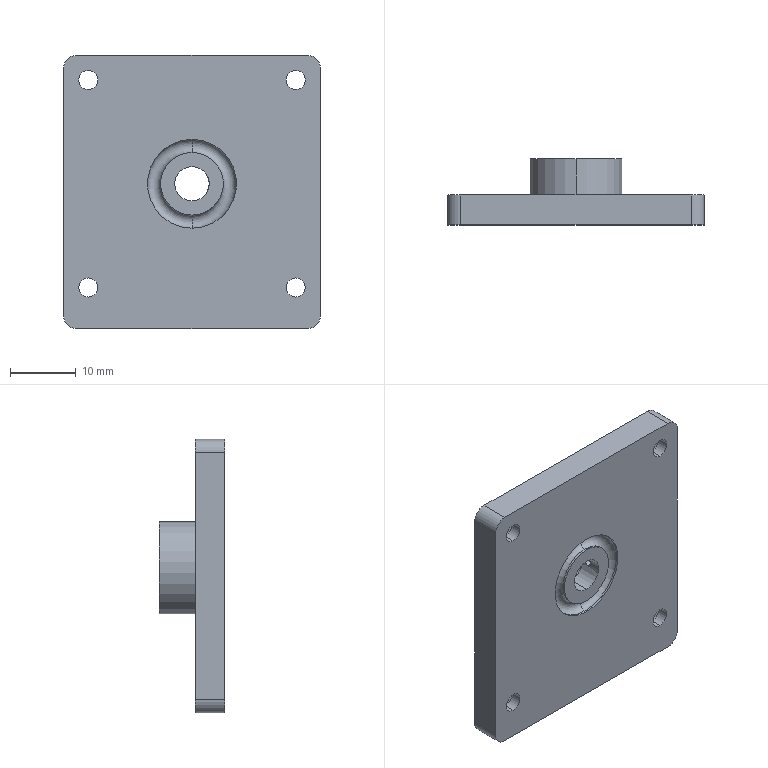Part | STEP file | 1 solid | 57 faces | box 39 x 10 x 41.5 mm | volume 7133 mm3 | cylinder 36 | plane 13 | cone 6 | torus 2 | commonest cylinder face diameters 2.9 x8 6 x8 4 x4 1.2 x2 2.5 x2 5.2 x2